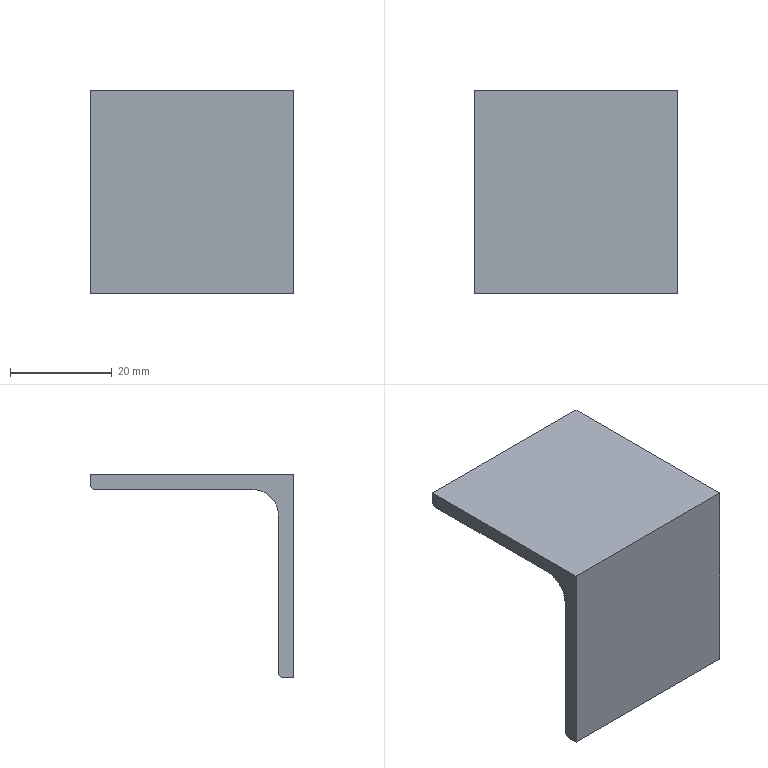Part | SolidWorks | features 3DProfileFeature 1, WeldMemberFeat 1, WeldmentFeature 1 | 1 solid | 11 faces | box 40 x 40 x 40 mm | volume 9437 mm3 | plane 8 | cylinder 3 | commonest cylinder face diameters 2 x2 10 x1
STEP:
#1=CARTESIAN_POINT('',(0.,0.,0.));
#2=VERTEX_POINT('',#1);
#3=CARTESIAN_POINT('',(0.,0.,-40.));
#4=VERTEX_POINT('',#3);
#5=CARTESIAN_POINT('',(0.,0.,-40.));
#6=DIRECTION('',(0.,0.,-1.));
#7=VECTOR('',#6,1000.);
#8=LINE('',#5,#7);
#9=EDGE_CURVE('',#2,#4,#8,.T.);
#10=ORIENTED_EDGE('',*,*,#9,.T.);
#11=CARTESIAN_POINT('',(40.,0.,-40.));
#12=VERTEX_POINT('',#11);
#13=CARTESIAN_POINT('',(40.,0.,-40.));
#14=DIRECTION('',(-1.,0.,0.));
#15=VECTOR('',#14,1000.);
#16=LINE('',#13,#15);
#17=EDGE_CURVE('',#12,#4,#16,.T.);
#18=ORIENTED_EDGE('',*,*,#17,.F.);
#19=CARTESIAN_POINT('',(40.,0.,0.));
#20=VERTEX_POINT('',#19);
#21=CARTESIAN_POINT('',(40.,0.,-40.));
#22=DIRECTION('',(0.,0.,-1.));
#23=VECTOR('',#22,1000.);
#24=LINE('',#21,#23);
#25=EDGE_CURVE('',#20,#12,#24,.T.);
#26=ORIENTED_EDGE('',*,*,#25,.F.);
#27=CARTESIAN_POINT('',(40.,0.,0.));
#28=DIRECTION('',(-1.,0.,0.));
#29=VECTOR('',#28,1000.);
#30=LINE('',#27,#29);
#31=EDGE_CURVE('',#20,#2,#30,.T.);
#32=ORIENTED_EDGE('',*,*,#31,.T.);
#33=EDGE_LOOP('',(#10,#18,#26,#32));
#34=FACE_OUTER_BOUND('',#33,.T.);
#35=CARTESIAN_POINT('',(40.,0.,-40.));
#36=DIRECTION('',(0.,1.,0.));
#37=DIRECTION('',(0.,0.,1.));
#38=AXIS2_PLACEMENT_3D('',#35,#36,#37);
#39=PLANE('',#38);
#40=ADVANCED_FACE('',(#34),#39,.F.);
#41=CARTESIAN_POINT('',(0.,2.,-40.));
#42=VERTEX_POINT('',#41);
#43=CARTESIAN_POINT('',(0.,0.,-40.));
#44=DIRECTION('',(0.,1.,0.));
#45=VECTOR('',#44,1000.);
#46=LINE('',#43,#45);
#47=EDGE_CURVE('',#4,#42,#46,.T.);
#48=ORIENTED_EDGE('',*,*,#47,.T.);
#49=CARTESIAN_POINT('',(40.,2.,-40.));
#50=VERTEX_POINT('',#49);
#51=CARTESIAN_POINT('',(40.,2.,-40.));
#52=DIRECTION('',(-1.,0.,0.));
#53=VECTOR('',#52,1000.);
#54=LINE('',#51,#53);
#55=EDGE_CURVE('',#50,#42,#54,.T.);
#56=ORIENTED_EDGE('',*,*,#55,.F.);
#57=CARTESIAN_POINT('',(40.,0.,-40.));
#58=DIRECTION('',(0.,1.,0.));
#59=VECTOR('',#58,1000.);
#60=LINE('',#57,#59);
#61=EDGE_CURVE('',#12,#50,#60,.T.);
#62=ORIENTED_EDGE('',*,*,#61,.F.);
#63=ORIENTED_EDGE('',*,*,#17,.T.);
#64=EDGE_LOOP('',(#48,#56,#62,#63));
#65=FACE_OUTER_BOUND('',#64,.T.);
#66=CARTESIAN_POINT('',(40.,0.,-40.));
#67=DIRECTION('',(0.,0.,1.));
#68=DIRECTION('',(1.,0.,0.));
#69=AXIS2_PLACEMENT_3D('',#66,#67,#68);
#70=PLANE('',#69);
#71=ADVANCED_FACE('',(#65),#70,.F.);
#72=CARTESIAN_POINT('',(0.,3.,-39.));
#73=VERTEX_POINT('',#72);
#74=CARTESIAN_POINT('',(0.,2.,-39.));
#75=DIRECTION('',(1.,0.,0.));
#76=DIRECTION('',(0.,0.,-1.));
#77=AXIS2_PLACEMENT_3D('',#74,#75,#76);
#78=CIRCLE('',#77,1.);
#79=EDGE_CURVE('',#42,#73,#78,.T.);
#80=ORIENTED_EDGE('',*,*,#79,.T.);
#81=CARTESIAN_POINT('',(40.,3.,-39.));
#82=VERTEX_POINT('',#81);
#83=CARTESIAN_POINT('',(40.,3.,-39.));
#84=DIRECTION('',(-1.,0.,0.));
#85=VECTOR('',#84,1000.);
#86=LINE('',#83,#85);
#87=EDGE_CURVE('',#82,#73,#86,.T.);
#88=ORIENTED_EDGE('',*,*,#87,.F.);
#89=CARTESIAN_POINT('',(40.,2.,-39.));
#90=DIRECTION('',(1.,0.,0.));
#91=DIRECTION('',(0.,0.,-1.));
#92=AXIS2_PLACEMENT_3D('',#89,#90,#91);
#93=CIRCLE('',#92,1.);
#94=EDGE_CURVE('',#50,#82,#93,.T.);
#95=ORIENTED_EDGE('',*,*,#94,.F.);
#96=ORIENTED_EDGE('',*,*,#55,.T.);
#97=EDGE_LOOP('',(#80,#88,#95,#96));
#98=FACE_OUTER_BOUND('',#97,.T.);
#99=CARTESIAN_POINT('',(40.,2.,-39.));
#100=DIRECTION('',(-1.,0.,0.));
#101=DIRECTION('',(0.,0.,1.));
#102=AXIS2_PLACEMENT_3D('',#99,#100,#101);
#103=CYLINDRICAL_SURFACE('',#102,1.);
#104=ADVANCED_FACE('',(#98),#103,.T.);
#105=CARTESIAN_POINT('',(0.,3.,-8.));
#106=VERTEX_POINT('',#105);
#107=CARTESIAN_POINT('',(0.,3.,-8.));
#108=DIRECTION('',(0.,0.,1.));
#109=VECTOR('',#108,1000.);
#110=LINE('',#107,#109);
#111=EDGE_CURVE('',#73,#106,#110,.T.);
#112=ORIENTED_EDGE('',*,*,#111,.T.);
#113=CARTESIAN_POINT('',(40.,3.,-8.));
#114=VERTEX_POINT('',#113);
#115=CARTESIAN_POINT('',(40.,3.,-8.));
#116=DIRECTION('',(-1.,0.,0.));
#117=VECTOR('',#116,1000.);
#118=LINE('',#115,#117);
#119=EDGE_CURVE('',#114,#106,#118,.T.);
#120=ORIENTED_EDGE('',*,*,#119,.F.);
#121=CARTESIAN_POINT('',(40.,3.,-8.));
#122=DIRECTION('',(0.,0.,1.));
#123=VECTOR('',#122,1000.);
#124=LINE('',#121,#123);
#125=EDGE_CURVE('',#82,#114,#124,.T.);
#126=ORIENTED_EDGE('',*,*,#125,.F.);
#127=ORIENTED_EDGE('',*,*,#87,.T.);
#128=EDGE_LOOP('',(#112,#120,#126,#127));
#129=FACE_OUTER_BOUND('',#128,.T.);
#130=CARTESIAN_POINT('',(40.,3.,-8.));
#131=DIRECTION('',(0.,-1.,0.));
#132=DIRECTION('',(0.,0.,-1.));
#133=AXIS2_PLACEMENT_3D('',#130,#131,#132);
#134=PLANE('',#133);
#135=ADVANCED_FACE('',(#129),#134,.F.);
#136=CARTESIAN_POINT('',(0.,8.,-3.));
#137=VERTEX_POINT('',#136);
#138=CARTESIAN_POINT('',(0.,8.,-8.));
#139=DIRECTION('',(-1.,0.,0.));
#140=DIRECTION('',(0.,0.,1.));
#141=AXIS2_PLACEMENT_3D('',#138,#139,#140);
#142=CIRCLE('',#141,5.);
#143=EDGE_CURVE('',#106,#137,#142,.T.);
#144=ORIENTED_EDGE('',*,*,#143,.T.);
#145=CARTESIAN_POINT('',(40.,8.,-3.));
#146=VERTEX_POINT('',#145);
#147=CARTESIAN_POINT('',(40.,8.,-3.));
#148=DIRECTION('',(-1.,0.,0.));
#149=VECTOR('',#148,1000.);
#150=LINE('',#147,#149);
#151=EDGE_CURVE('',#146,#137,#150,.T.);
#152=ORIENTED_EDGE('',*,*,#151,.F.);
#153=CARTESIAN_POINT('',(40.,8.,-8.));
#154=DIRECTION('',(-1.,0.,0.));
#155=DIRECTION('',(0.,0.,1.));
#156=AXIS2_PLACEMENT_3D('',#153,#154,#155);
#157=CIRCLE('',#156,5.);
#158=EDGE_CURVE('',#114,#146,#157,.T.);
#159=ORIENTED_EDGE('',*,*,#158,.F.);
#160=ORIENTED_EDGE('',*,*,#119,.T.);
#161=EDGE_LOOP('',(#144,#152,#159,#160));
#162=FACE_OUTER_BOUND('',#161,.T.);
#163=CARTESIAN_POINT('',(40.,8.,-8.));
#164=DIRECTION('',(-1.,0.,0.));
#165=DIRECTION('',(0.,0.,1.));
#166=AXIS2_PLACEMENT_3D('',#163,#164,#165);
#167=CYLINDRICAL_SURFACE('',#166,5.);
#168=ADVANCED_FACE('',(#162),#167,.F.);
#169=CARTESIAN_POINT('',(0.,39.,-3.));
#170=VERTEX_POINT('',#169);
#171=CARTESIAN_POINT('',(0.,39.,-3.));
#172=DIRECTION('',(0.,1.,0.));
#173=VECTOR('',#172,1000.);
#174=LINE('',#171,#173);
#175=EDGE_CURVE('',#137,#170,#174,.T.);
#176=ORIENTED_EDGE('',*,*,#175,.T.);
#177=CARTESIAN_POINT('',(40.,39.,-3.));
#178=VERTEX_POINT('',#177);
#179=CARTESIAN_POINT('',(40.,39.,-3.));
#180=DIRECTION('',(-1.,0.,0.));
#181=VECTOR('',#180,1000.);
#182=LINE('',#179,#181);
#183=EDGE_CURVE('',#178,#170,#182,.T.);
#184=ORIENTED_EDGE('',*,*,#183,.F.);
#185=CARTESIAN_POINT('',(40.,39.,-3.));
#186=DIRECTION('',(0.,1.,0.));
#187=VECTOR('',#186,1000.);
#188=LINE('',#185,#187);
#189=EDGE_CURVE('',#146,#178,#188,.T.);
#190=ORIENTED_EDGE('',*,*,#189,.F.);
#191=ORIENTED_EDGE('',*,*,#151,.T.);
#192=EDGE_LOOP('',(#176,#184,#190,#191));
#193=FACE_OUTER_BOUND('',#192,.T.);
#194=CARTESIAN_POINT('',(40.,39.,-3.));
#195=DIRECTION('',(0.,0.,1.));
#196=DIRECTION('',(0.,-1.,0.));
#197=AXIS2_PLACEMENT_3D('',#194,#195,#196);
#198=PLANE('',#197);
#199=ADVANCED_FACE('',(#193),#198,.F.);
#200=CARTESIAN_POINT('',(0.,40.,-2.));
#201=VERTEX_POINT('',#200);
#202=CARTESIAN_POINT('',(0.,39.,-2.));
#203=DIRECTION('',(1.,0.,0.));
#204=DIRECTION('',(0.,0.,1.));
#205=AXIS2_PLACEMENT_3D('',#202,#203,#204);
#206=CIRCLE('',#205,1.);
#207=EDGE_CURVE('',#170,#201,#206,.T.);
#208=ORIENTED_EDGE('',*,*,#207,.T.);
#209=CARTESIAN_POINT('',(40.,40.,-2.));
#210=VERTEX_POINT('',#209);
#211=CARTESIAN_POINT('',(40.,40.,-2.));
#212=DIRECTION('',(-1.,0.,0.));
#213=VECTOR('',#212,1000.);
#214=LINE('',#211,#213);
#215=EDGE_CURVE('',#210,#201,#214,.T.);
#216=ORIENTED_EDGE('',*,*,#215,.F.);
#217=CARTESIAN_POINT('',(40.,39.,-2.));
#218=DIRECTION('',(1.,0.,0.));
#219=DIRECTION('',(0.,0.,1.));
#220=AXIS2_PLACEMENT_3D('',#217,#218,#219);
#221=CIRCLE('',#220,1.);
#222=EDGE_CURVE('',#178,#210,#221,.T.);
#223=ORIENTED_EDGE('',*,*,#222,.F.);
#224=ORIENTED_EDGE('',*,*,#183,.T.);
#225=EDGE_LOOP('',(#208,#216,#223,#224));
#226=FACE_OUTER_BOUND('',#225,.T.);
#227=CARTESIAN_POINT('',(40.,39.,-2.));
#228=DIRECTION('',(-1.,0.,0.));
#229=DIRECTION('',(0.,0.,1.));
#230=AXIS2_PLACEMENT_3D('',#227,#228,#229);
#231=CYLINDRICAL_SURFACE('',#230,1.);
#232=ADVANCED_FACE('',(#226),#231,.T.);
#233=CARTESIAN_POINT('',(0.,40.,0.));
#234=VERTEX_POINT('',#233);
#235=CARTESIAN_POINT('',(0.,40.,0.));
#236=DIRECTION('',(0.,0.,1.));
#237=VECTOR('',#236,1000.);
#238=LINE('',#235,#237);
#239=EDGE_CURVE('',#201,#234,#238,.T.);
#240=ORIENTED_EDGE('',*,*,#239,.T.);
#241=CARTESIAN_POINT('',(40.,40.,0.));
#242=VERTEX_POINT('',#241);
#243=CARTESIAN_POINT('',(40.,40.,0.));
#244=DIRECTION('',(-1.,0.,0.));
#245=VECTOR('',#244,1000.);
#246=LINE('',#243,#245);
#247=EDGE_CURVE('',#242,#234,#246,.T.);
#248=ORIENTED_EDGE('',*,*,#247,.F.);
#249=CARTESIAN_POINT('',(40.,40.,0.));
#250=DIRECTION('',(0.,0.,1.));
#251=VECTOR('',#250,1000.);
#252=LINE('',#249,#251);
#253=EDGE_CURVE('',#210,#242,#252,.T.);
#254=ORIENTED_EDGE('',*,*,#253,.F.);
#255=ORIENTED_EDGE('',*,*,#215,.T.);
#256=EDGE_LOOP('',(#240,#248,#254,#255));
#257=FACE_OUTER_BOUND('',#256,.T.);
#258=CARTESIAN_POINT('',(40.,40.,0.));
#259=DIRECTION('',(0.,-1.,0.));
#260=DIRECTION('',(0.,0.,-1.));
#261=AXIS2_PLACEMENT_3D('',#258,#259,#260);
#262=PLANE('',#261);
#263=ADVANCED_FACE('',(#257),#262,.F.);
#264=CARTESIAN_POINT('',(0.,0.,0.));
#265=DIRECTION('',(0.,-1.,0.));
#266=VECTOR('',#265,1000.);
#267=LINE('',#264,#266);
#268=EDGE_CURVE('',#234,#2,#267,.T.);
#269=ORIENTED_EDGE('',*,*,#268,.T.);
#270=ORIENTED_EDGE('',*,*,#31,.F.);
#271=CARTESIAN_POINT('',(40.,0.,0.));
#272=DIRECTION('',(0.,-1.,0.));
#273=VECTOR('',#272,1000.);
#274=LINE('',#271,#273);
#275=EDGE_CURVE('',#242,#20,#274,.T.);
#276=ORIENTED_EDGE('',*,*,#275,.F.);
#277=ORIENTED_EDGE('',*,*,#247,.T.);
#278=EDGE_LOOP('',(#269,#270,#276,#277));
#279=FACE_OUTER_BOUND('',#278,.T.);
#280=CARTESIAN_POINT('',(40.,0.,0.));
#281=DIRECTION('',(0.,0.,-1.));
#282=DIRECTION('',(-1.,0.,0.));
#283=AXIS2_PLACEMENT_3D('',#280,#281,#282);
#284=PLANE('',#283);
#285=ADVANCED_FACE('',(#279),#284,.F.);
#286=ORIENTED_EDGE('',*,*,#25,.T.);
#287=ORIENTED_EDGE('',*,*,#61,.T.);
#288=ORIENTED_EDGE('',*,*,#94,.T.);
#289=ORIENTED_EDGE('',*,*,#125,.T.);
#290=ORIENTED_EDGE('',*,*,#158,.T.);
#291=ORIENTED_EDGE('',*,*,#189,.T.);
#292=ORIENTED_EDGE('',*,*,#222,.T.);
#293=ORIENTED_EDGE('',*,*,#253,.T.);
#294=ORIENTED_EDGE('',*,*,#275,.T.);
#295=EDGE_LOOP('',(#286,#287,#288,#289,#290,#291,#292,#293,#294));
#296=FACE_OUTER_BOUND('',#295,.T.);
#297=CARTESIAN_POINT('',(40.,39.,-2.));
#298=DIRECTION('',(-1.,0.,0.));
#299=DIRECTION('',(0.,0.,1.));
#300=AXIS2_PLACEMENT_3D('',#297,#298,#299);
#301=PLANE('',#300);
#302=ADVANCED_FACE('',(#296),#301,.F.);
#303=ORIENTED_EDGE('',*,*,#9,.F.);
#304=ORIENTED_EDGE('',*,*,#268,.F.);
#305=ORIENTED_EDGE('',*,*,#239,.F.);
#306=ORIENTED_EDGE('',*,*,#207,.F.);
#307=ORIENTED_EDGE('',*,*,#175,.F.);
#308=ORIENTED_EDGE('',*,*,#143,.F.);
#309=ORIENTED_EDGE('',*,*,#111,.F.);
#310=ORIENTED_EDGE('',*,*,#79,.F.);
#311=ORIENTED_EDGE('',*,*,#47,.F.);
#312=EDGE_LOOP('',(#303,#304,#305,#306,#307,#308,#309,#310,#311));
#313=FACE_OUTER_BOUND('',#312,.T.);
#314=CARTESIAN_POINT('',(0.,39.,-2.));
#315=DIRECTION('',(-1.,0.,0.));
#316=DIRECTION('',(0.,0.,1.));
#317=AXIS2_PLACEMENT_3D('',#314,#315,#316);
#318=PLANE('',#317);
#319=ADVANCED_FACE('',(#313),#318,.T.);
#320=CLOSED_SHELL('',(#40,#71,#104,#135,#168,#199,#232,#263,#285,#302,#319));
#321=MANIFOLD_SOLID_BREP('',#320);
#322=CARTESIAN_POINT('',(0.,0.,0.));
#323=DIRECTION('',(0.,0.,1.));
#324=DIRECTION('',(1.,0.,0.));
#325=AXIS2_PLACEMENT_3D('',#322,#323,#324);
#326=(LENGTH_UNIT()NAMED_UNIT(*)SI_UNIT(.MILLI.,.METRE.));
#327=UNCERTAINTY_MEASURE_WITH_UNIT(LENGTH_MEASURE(0.00001),#326,'','');
#328=(NAMED_UNIT(*)PLANE_ANGLE_UNIT()SI_UNIT($,.RADIAN.));
#329=(NAMED_UNIT(*)SI_UNIT($,.STERADIAN.)SOLID_ANGLE_UNIT());
#330=(GEOMETRIC_REPRESENTATION_CONTEXT(3)GLOBAL_UNCERTAINTY_ASSIGNED_CONTEXT((#327))GLOBAL_UNIT_ASSIGNED_CONTEXT((#326,#328,#329))REPRESENTATION_CONTEXT('',''));
#331=ADVANCED_BREP_SHAPE_REPRESENTATION('',(#321,#325),#330);